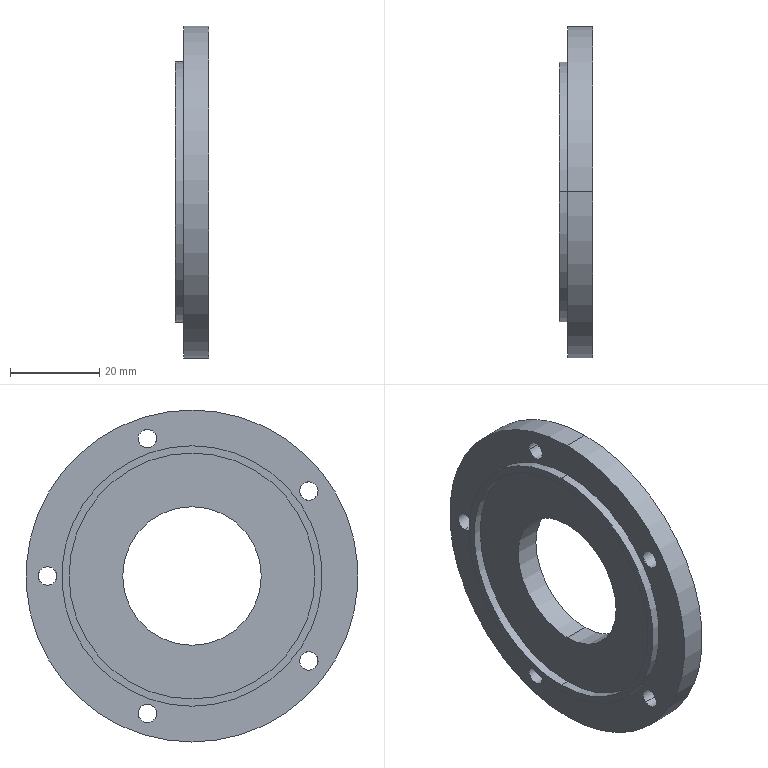Part | STEP file | Completa.sldasm-Part-20_Valor predeterminado | 1 solid | 42 faces | box 7.542 x 74.256 x 74.256 mm | volume 20001 mm3 | cylinder 28 | cone 10 | plane 4 | commonest cylinder face diameters 4.117 x10 7.53 x10 31 x2 55 x2 58.256 x2 74.256 x2